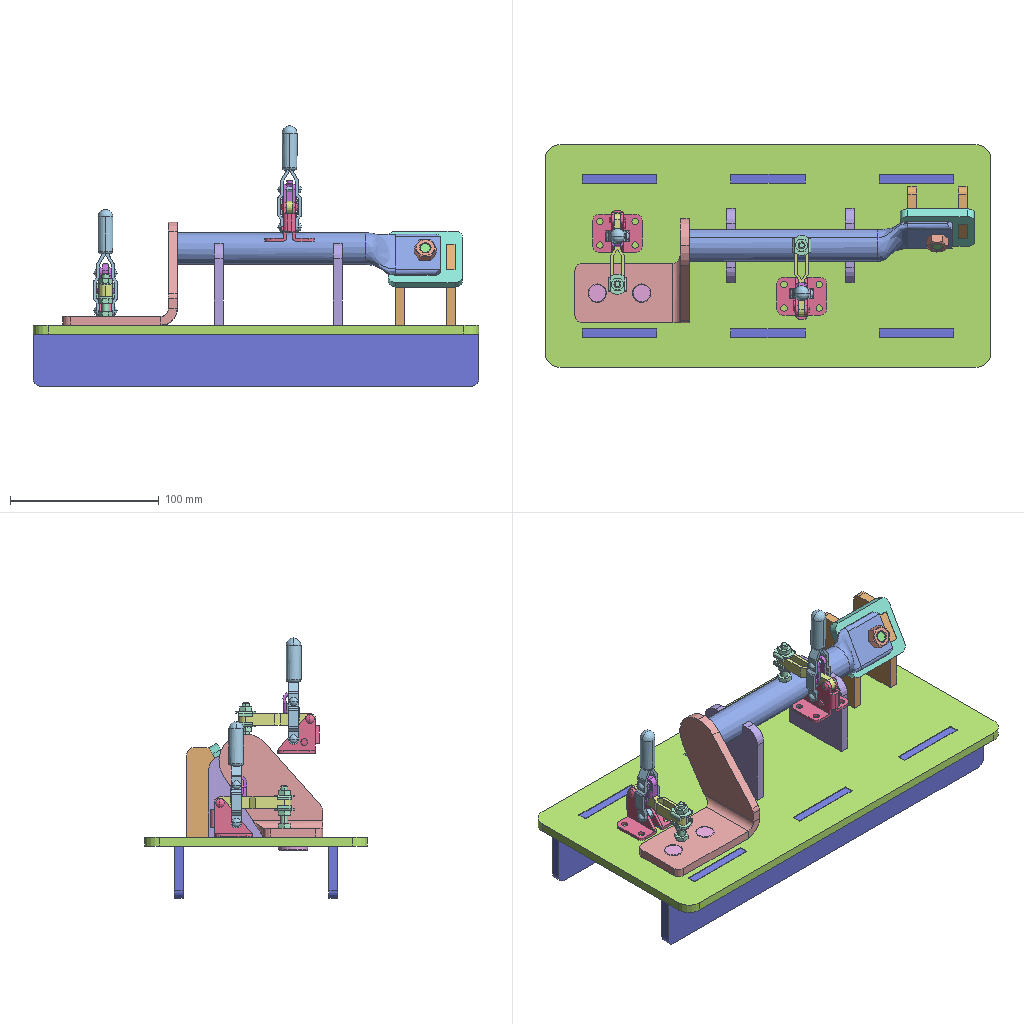Assembly | SolidWorks | 11 different items | 16 placed | box 300 x 150 x 175 mm
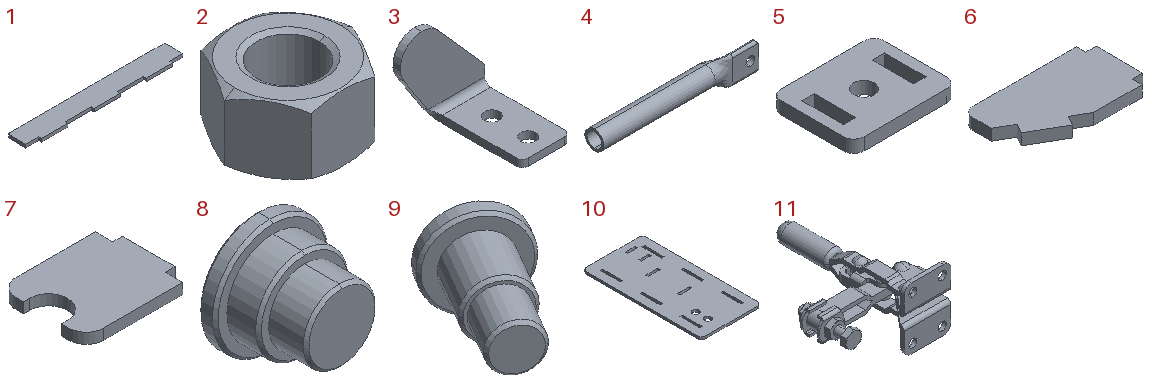Parts list (item | quantity | size | volume | features):
1 | x2 | 300 x 40.5 x 6 mm | 67886 mm3 | features FlatPattern 1, SMBaseFlange 1, SheetMetal 1
2 | x1 | 27.713 x 24 x 14.8 mm | 5071 mm3 | features RevCut 2, Chamfer 1, Extrusion 1, LPattern 1
3 | x1 | 70 x 77 x 69.5 mm | 32666 mm3 | features ICE 2, Fillet 1, FlatPattern 1, SMBaseFlange 1, SheetMetal 1
4 | x1 | 177 x 21.701 x 31 mm | 30996 mm3 | features ICE 3, Chamfer 2, Blend 1, ExtruThin 1
5 | x1 | 50 x 40 x 6 mm | 9960 mm3 | features FlatPattern 1, SMBaseFlange 1, SheetMetal 1
6 | x2 | 65.896 x 35.023 x 6 mm | 12093 mm3 | features FlatPattern 1, SMBaseFlange 1, SheetMetal 1
7 | x2 | 60.5 x 50 x 6 mm | 15667 mm3 | features FlatPattern 1, SMBaseFlange 1, SheetMetal 1
8 | x2 | 20 x 15 x 20 mm | 2820 mm3 | features Chamfer 1, Revolution 1
9 | x1 | 19.959 x 23.437 x 15 mm | 1699 mm3 | features Chamfer 1, Revolution 1
10 | x1 | 150 x 300 x 6 mm | 252312 mm3 | features FlatPattern 1, SMBaseFlange 1, SheetMetal 1
11 | x2 | 56.45 x 77.62 x 33.3 mm | 10418 mm3 | features BaseBody 5
Mates (type | each side: item.copy, entity, surface, feature):
Coincident | 3.1 face plane Base-Flange1 | 4.1 face plane Extrude-Thin1
Concentric | 3.1 face cylinder Cut-Extrude2 | 4.1 face cylinder Extrude-Thin1
PlanarAngleDim | 4.1 face plane Boss-Extrude1 | 3.1 face plane Base-Flange1
InPlace | 3.1 face plane Base-Flange1 | 10.1 plane
InPlace | 8.1 plane | assembly plane
InPlace | 4.1 face plane Boss-Extrude1 | 5.1 plane
InPlace | 6.1 plane | assembly plane
InPlace | 7.1 plane | assembly plane
InPlace | 9.1 plane | assembly plane
Coincident | 3.1 face plane Base-Flange1 | 11.1 face plane PN_0001 vertical flange quick clamp [PN_0002] (bolt) solid1
DistanceDim | 11.1 face plane PN_0001 vertical flange quick clamp [PN_0002] (bolt) solid1 | 3.1 face plane Cut-Extrude2
DistanceDim | 11.1 face plane PN_0001 vertical flange quick clamp [PN_0002] (seat) solid1 | 3.1 face plane Base-Flange1
Coincident | 4.1 face plane Boss-Extrude1 | 2.1 face plane BaseNut
Concentric | 9.1 face cylinder Revolve1 | 2.1 edge
Tangent | 4.1 face cylinder Extrude-Thin1 | 11.2 face plane PN_0001 vertical flange quick clamp [PN_0002] (bolt) solid1
Parallel | 7.1 face plane Base-Flange1 | 11.2 face plane PN_0001 vertical flange quick clamp [PN_0002] (seat) solid1
DistanceDim | 11.2 face plane PN_0001 vertical flange quick clamp [PN_0002] (seat) solid1 | 3.1 face plane Base-Flange1
DistanceDim | 11.2 face plane PN_0001 vertical flange quick clamp [PN_0002] (bolt) solid1 | 4.1 face cylinder Extrude-Thin1
InPlace | 1.1 plane | assembly plane